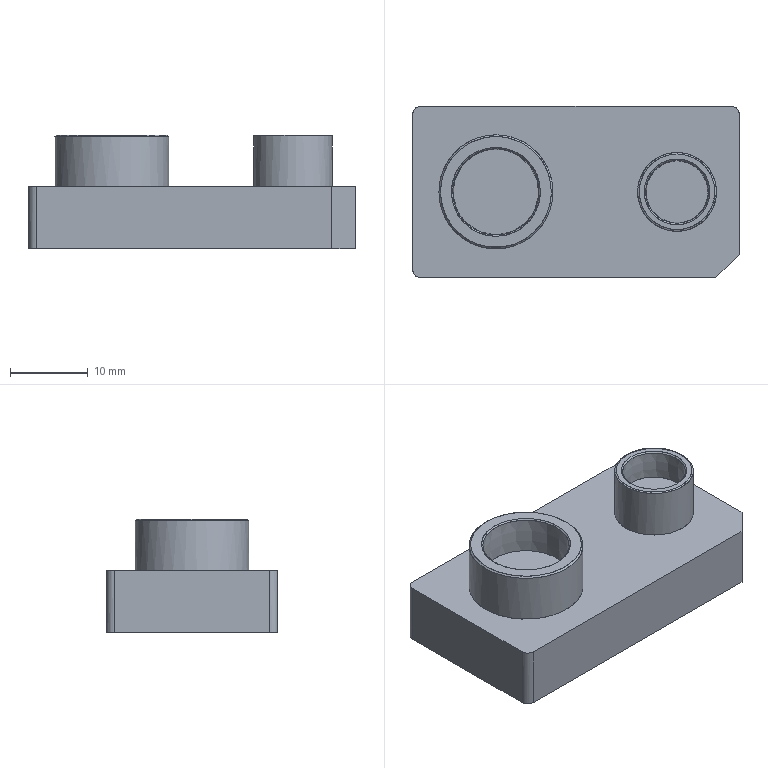NC program | PowerMill | posted by the shop | part box 42 x 22 x 14.621 mm
Lines 13250 to 14233 of 126517:
( TOOL ID   D10_1_1 )
( TOOL DIA. 10. TIP RAD 0 LENGTH 69.8 )
( Z = -.269 )
T3 M6
T14
G91 G28 Z0
G0 G90 G54
M08
S8500 M3
X0 Y0 M8
G43 Z11.801 H3
X-28.191 Y.483
Z.931
G1 Z-.269 F360
X-22.918 Y.327 F600
X-9.229 Y-12.572
G3 X-8.361 Y-12.468 I-1.292 J14.426
G1 X-8.126 Y-12.428
X-7.724 Y-12.351
X-7.405 Y-12.28
X-7.078 Y-12.198
X-6.754 Y-12.109
X-6.129 Y-11.908
X-5.492 Y-11.665
X-5.051 Y-11.472
X-4.855 Y-11.381
X-4.533 Y-11.219
X-21.847 Y5.097
X-21.746 Y5.321
X-21.544 Y5.734
X-21.428 Y5.955
X-21.195 Y6.374
X-21.109 Y6.516
X-20.794 Y7.013
X-20.47 Y7.475
X-20.089 Y7.968
X-19.835 Y8.267
X-19.487 Y8.652
X-1.123 Y-8.653
X-.713 Y-8.199
X-.395 Y-7.812
X-.268 Y-7.647
X-.032 Y-7.328
X.241 Y-6.93
X.403 Y-6.674
X.561 Y-6.416
X.766 Y-6.056
X.932 Y-5.738
X1.092 Y-5.416
X1.237 Y-5.099
X-16.078 Y11.219
X-15.693 Y11.408
X-15.371 Y11.557
X-14.797 Y11.792
X-14.418 Y11.927
X-14.1 Y12.034
X-13.782 Y12.128
X-13.463 Y12.216
X-13.143 Y12.294
X-12.821 Y12.365
X-12.184 Y12.478
X-11.547 Y12.557
X-11.379 Y12.57
X2.309 Y-.33
G0 Z4.001
G1 X28.324 Y-3.114 F10000
G0 Z.931
G1 Z-.269 F360
X23.158 Y-2.05 F600
X12.123 Y10.326
X11.843 Y10.299
X11.524 Y10.258
X11.204 Y10.207
X10.885 Y10.145
X10.566 Y10.074
X10.247 Y9.992
X9.919 Y9.895
X9.608 Y9.793
X9.289 Y9.677
X9.037 Y9.576
X8.65 Y9.408
X8.332 Y9.252
X8.012 Y9.085
X7.79 Y8.957
X21.303 Y-6.198
X21.1 Y-6.466
X20.782 Y-6.846
X20.622 Y-7.022
X20.314 Y-7.343
X20.145 Y-7.507
X19.824 Y-7.801
X19.609 Y-7.982
X19.205 Y-8.301
X18.866 Y-8.544
X18.547 Y-8.756
X18.211 Y-8.959
X4.696 Y6.199
X4.595 Y6.064
X4.374 Y5.744
X4.182 Y5.444
X3.98 Y5.106
X3.809 Y4.787
X3.648 Y4.467
X3.503 Y4.149
X3.369 Y3.829
X3.225 Y3.444
X3.139 Y3.191
X3.042 Y2.872
X2.955 Y2.552
X2.88 Y2.233
X2.842 Y2.05
X13.876 Y-10.326
G0 Z11.801
X0 Y0
Z9.801
X1.258 Y-21.755
Z-5.62
G1 Z-6.82 F360
Y-16.48 F600
X1.136 Y-5.545
X.851 Y-6.099
X.787 Y-6.215
X.451 Y-6.779
X.268 Y-7.062
X.073 Y-7.344
X-.284 Y-7.825
X-.581 Y-8.192
X-.827 Y-8.474
X-1.1 Y-8.77
X-1.418 Y-9.093
X-1.696 Y-9.356
X-1.974 Y-9.604
X-2.27 Y-9.853
X-2.674 Y-10.169
X-3.121 Y-10.49
X-3.491 Y-10.734
X-3.688 Y-10.857
X-4.255 Y-11.183
X-4.476 Y-11.299
X-4.823 Y-11.472
X-5.39 Y-11.726
X-5.735 Y-11.864
X-5.958 Y-11.947
X-6.525 Y-12.139
X-7.092 Y-12.301
X-7.66 Y-12.436
X-8.227 Y-12.543
X-8.795 Y-12.624
X-9.362 Y-12.679
X-9.929 Y-12.708
X-10.497 Y-12.712
X-11.064 Y-12.691
X-11.632 Y-12.644
X-12.199 Y-12.572
X-12.766 Y-12.473
X-12.98 Y-12.429
X-13.334 Y-12.348
X-13.901 Y-12.195
X-14.469 Y-12.013
X-14.874 Y-11.864
X-15.036 Y-11.8
X-15.603 Y-11.557
X-16.171 Y-11.28
X-16.738 Y-10.966
X-17.117 Y-10.734
X-17.305 Y-10.613
X-17.589 Y-10.42
X-17.935 Y-10.169
X-18.44 Y-9.77
X-18.697 Y-9.55
X-19.008 Y-9.268
X-19.245 Y-9.039
X-19.546 Y-8.731
X-19.782 Y-8.474
X-20.142 Y-8.053
X-20.477 Y-7.627
X-20.71 Y-7.305
X-21.06 Y-6.779
X-21.277 Y-6.422
X-21.396 Y-6.215
X-21.694 Y-5.65
X-21.829 Y-5.369
X-21.957 Y-5.085
X-22.188 Y-4.52
X-22.412 Y-3.879
X-22.558 Y-3.39
X-22.7 Y-2.825
X-22.816 Y-2.26
X-22.905 Y-1.695
X-22.968 Y-1.13
X-23.006 Y-.565
X-23.018 Y0
X-23.006 Y.565
X-22.968 Y1.13
X-22.905 Y1.695
X-22.816 Y2.26
X-22.7 Y2.825
X-22.558 Y3.39
X-22.388 Y3.955
X-22.188 Y4.52
X-21.957 Y5.085
X-21.829 Y5.369
X-21.694 Y5.65
X-21.396 Y6.215
X-21.277 Y6.422
X-21.06 Y6.779
X-20.682 Y7.344
X-20.477 Y7.627
X-20.142 Y8.053
X-19.782 Y8.474
X-19.546 Y8.731
X-19.245 Y9.039
X-19.008 Y9.268
X-18.635 Y9.604
X-18.44 Y9.77
X-17.873 Y10.216
X-17.589 Y10.42
X-17.305 Y10.613
X-17.117 Y10.734
X-16.738 Y10.966
X-16.133 Y11.299
X-15.603 Y11.557
X-15.036 Y11.801
X-14.874 Y11.864
X-14.469 Y12.013
X-13.901 Y12.195
X-13.334 Y12.348
X-12.98 Y12.429
X-12.766 Y12.473
X-12.199 Y12.572
X-11.632 Y12.645
X-11.064 Y12.691
X-10.497 Y12.712
X-9.929 Y12.708
X-9.362 Y12.679
X-8.795 Y12.624
X-8.227 Y12.543
X-7.63 Y12.429
X-7.092 Y12.301
X-6.525 Y12.139
X-5.958 Y11.948
X-5.735 Y11.864
X-5.39 Y11.726
X-4.823 Y11.472
X-4.476 Y11.299
X-4.255 Y11.183
X-3.688 Y10.857
X-3.491 Y10.734
X-3.121 Y10.49
X-2.674 Y10.169
X-2.27 Y9.853
X-1.974 Y9.604
X-1.696 Y9.356
X-1.364 Y9.039
X-1.1 Y8.77
X-.827 Y8.474
X-.581 Y8.192
X-.284 Y7.825
X.073 Y7.344
X.268 Y7.062
X.451 Y6.779
X.624 Y6.497
X.851 Y6.097
X1.085 Y5.65
G2 X1.418 Y4.921 I-11.182 J-5.554
G1 X1.579 Y4.52
X1.779 Y3.955
X1.949 Y3.39
X2.092 Y2.825
X2.207 Y2.26
X2.296 Y1.695
X2.359 Y1.13
X2.397 Y.565
X2.409 Y0
X2.397 Y-.565
X2.359 Y-1.13
X2.296 Y-1.695
X2.207 Y-2.26
X2.092 Y-2.825
X1.949 Y-3.39
X1.779 Y-3.955
X1.579 Y-4.52
X1.418 Y-4.921
X1.282 Y-5.235
X1.136 Y-5.545
X.548 Y-6.8
X.438 Y-6.998 Z-6.818
X.302 Y-7.178 Z-6.811
X-.628 Y-8.247 Z-6.755
X-.637 Y-8.257 Z-6.748
Z-6.727
X-.628 Y-8.246 Z-6.72
X-.581 Y-8.192 Z-6.721 F360
X-.35 Y-7.909 Z-6.728
X-.284 Y-7.825 Z-6.729
X.073 Y-7.344 Z-6.74
X.268 Y-7.062 Z-6.746
X.451 Y-6.779 Z-6.752
X.787 Y-6.215 Z-6.763
X.851 Y-6.099 Z-6.766
X1.085 Y-5.65 Z-6.774
X1.258 Y-5.288 Z-6.781
X1.418 Y-4.921 Z-6.788
X1.579 Y-4.52 Z-6.796
X1.779 Y-3.955 Z-6.806
X1.949 Y-3.39 Z-6.817
X1.986 Y-3.254 Z-6.819
X1.997 Y-3.207 Z-6.82
X3.536 Y-4.437 F600
X3.443 Y-4.237
X3.323 Y-3.955
X3.111 Y-3.39
X2.935 Y-2.825
X2.793 Y-2.26
X2.735 Y-1.977
X2.685 Y-1.695
X2.642 Y-1.412
X2.608 Y-1.13
X2.562 Y-.565
X2.553 Y-.377
X2.546 Y0
X2.553 Y.377
X2.562 Y.565
X2.608 Y1.13
X2.642 Y1.412
X2.685 Y1.695
X2.735 Y1.977
X2.793 Y2.26
X2.935 Y2.825
X3.121 Y3.417
X3.323 Y3.955
X3.443 Y4.237
X3.574 Y4.52
X3.714 Y4.802
X3.866 Y5.085
X4.029 Y5.367
X4.255 Y5.728
X4.382 Y5.916
X4.594 Y6.215
X4.823 Y6.512
X5.043 Y6.779
X5.39 Y7.167
X5.561 Y7.344
X5.958 Y7.726
X6.165 Y7.909
X6.525 Y8.207
X6.809 Y8.423
X7.092 Y8.624
X7.376 Y8.812
X7.749 Y9.039
X8.227 Y9.301
X8.511 Y9.441
X8.873 Y9.604
X9.362 Y9.8
X9.929 Y9.993
X10.578 Y10.169
X11.064 Y10.273
X11.632 Y10.364
X12.199 Y10.423
X12.766 Y10.451
X13.334 Y10.448
X13.901 Y10.415
X14.469 Y10.35
X15.036 Y10.254
X15.422 Y10.169
X15.603 Y10.125
X15.887 Y10.047
X16.171 Y9.961
X16.738 Y9.762
X17.127 Y9.604
X17.305 Y9.526
X17.589 Y9.393
X17.873 Y9.249
X18.251 Y9.039
X18.44 Y8.926
X18.724 Y8.748
X19.121 Y8.474
X19.264 Y8.369
X19.575 Y8.127
X19.859 Y7.889
X20.142 Y7.633
X20.439 Y7.344
X20.71 Y7.06
X20.957 Y6.779
X21.199 Y6.485
X21.406 Y6.215
X21.607 Y5.932
X21.845 Y5.572
X22.134 Y5.085
X22.285 Y4.802
X22.426 Y4.52
X22.677 Y3.955
X22.889 Y3.39
X22.979 Y3.112
X23.065 Y2.825
X23.207 Y2.26
X23.265 Y1.977
X23.315 Y1.695
X23.358 Y1.412
X23.392 Y1.13
X23.438 Y.565
X23.454 Y0
X23.438 Y-.565
X23.392 Y-1.13
X23.358 Y-1.412
X23.315 Y-1.695
X23.265 Y-1.977
X23.207 Y-2.26
X23.065 Y-2.825
X22.979 Y-3.112
X22.889 Y-3.39
X22.677 Y-3.955
X22.557 Y-4.237
X22.426 Y-4.52
X22.285 Y-4.802
X22.134 Y-5.085
X21.845 Y-5.573
X21.607 Y-5.932
X21.406 Y-6.215
X21.277 Y-6.385
X20.957 Y-6.779
X20.708 Y-7.062
X20.439 Y-7.344
X20.142 Y-7.633
X19.835 Y-7.909
X19.575 Y-8.127
X19.348 Y-8.306
X19.008 Y-8.555
X18.724 Y-8.747
X18.44 Y-8.926
X18.251 Y-9.039
X17.873 Y-9.249
X17.589 Y-9.393
X17.305 Y-9.526
X17.128 Y-9.604
X16.738 Y-9.762
X16.454 Y-9.867
X16.172 Y-9.961
X15.887 Y-10.047
X15.603 Y-10.125
X15.422 Y-10.169
X15.036 Y-10.254
X14.469 Y-10.35
X13.901 Y-10.415
X13.334 Y-10.448
X13.05 Y-10.454
X12.766 Y-10.451
X12.199 Y-10.423
X11.632 Y-10.364
X11.064 Y-10.273
X10.497 Y-10.15
X9.929 Y-9.993
X9.362 Y-9.8
X8.795 Y-9.571
X8.511 Y-9.441
X8.227 Y-9.301
X7.749 Y-9.039
X7.376 Y-8.812
X7.092 Y-8.624
X6.809 Y-8.423
X6.525 Y-8.207
X6.165 Y-7.909
X5.958 Y-7.726
X5.561 Y-7.344
X5.39 Y-7.167
X5.043 Y-6.779
X4.823 Y-6.513
X4.594 Y-6.215
X4.42 Y-5.971
X4.204 Y-5.65
X4.029 Y-5.367
X3.866 Y-5.085
X3.714 Y-4.802
X3.536 Y-4.437
G0 Z9.801
X0 Y0
X25.992 Y-17.264
Z-13.52
G1 Z-14.72 F360
G3 X22.456 Y-13.728 I-1.768 J1.768 F600
G1 X21.585 Y-14.599
X21.584 Y-14.6
X21.583 Y-14.601
X21.395 Y-14.779
X21.393 Y-14.78
X21.392 Y-14.782
X21.232 Y-14.919
X21.23 Y-14.921
X21.229 Y-14.922
X21.073 Y-15.045
X21.072 Y-15.046
X21.07 Y-15.047
X20.797 Y-15.24
X20.795 Y-15.242
X20.792 Y-15.244
X20.433 Y-15.46
X20.43 Y-15.461
X20.428 Y-15.462
X20.234 Y-15.562
X20.233 Y-15.563
X20.232
X20.109 Y-15.621
X20.108 Y-15.622
X20.106 Y-15.623
X19.79 Y-15.754
X19.787 Y-15.755
X19.784 Y-15.756
X19.4 Y-15.883
X19.397 Y-15.884
X19.395 Y-15.885
X19.147 Y-15.949
X19.145
X19.142 Y-15.95
X18.826 Y-16.012
X18.824 Y-16.013
X18.821
X18.505 Y-16.055
X18.502
X18.5
X18.184 Y-16.077
X18.181
X18.179
X17.863 Y-16.08
X17.862
X-20.075 Y-16.079
X-20.077
X-20.078
X-20.394 Y-16.067
X-20.397
X-20.399
X-20.715 Y-16.038
X-20.717 Y-16.037
X-20.719
X-21.035 Y-15.991
X-21.037
X-21.039 Y-15.99
X-21.356 Y-15.927
X-21.358 Y-15.926
X-21.36
X-21.676 Y-15.844
X-21.678
X-21.68 Y-15.843
X-21.996 Y-15.743
X-21.998 Y-15.742
X-22.001 Y-15.741
X-22.317 Y-15.621
X-22.319 Y-15.62
X-22.321
X-22.637 Y-15.478
X-22.639 Y-15.477
X-22.641 Y-15.476
X-22.957 Y-15.312
X-22.959 Y-15.311
X-22.96
X-23.076 Y-15.244
X-23.077
X-23.078 Y-15.243
X-23.279 Y-15.12
X-23.28 Y-15.119
X-23.282 Y-15.118
X-23.565 Y-14.925
X-23.567 Y-14.923
X-23.569 Y-14.922
X-23.918 Y-14.649
X-23.921 Y-14.647
X-23.923 Y-14.645
X-24.239 Y-14.359
X-24.24 Y-14.357
X-24.241 Y-14.356
X-24.315 Y-14.283
X-24.316 Y-14.282
X-24.317 Y-14.281
X-24.56 Y-14.022
X-24.562 Y-14.02
X-24.563 Y-14.018
X-24.866 Y-13.645
X-24.868 Y-13.642
X-24.87 Y-13.64
X-25.09 Y-13.324
X-25.091 Y-13.322
X-25.092 Y-13.321
X-25.201 Y-13.149
X-25.202 Y-13.147
X-25.203 Y-13.146
X-25.287 Y-13.002
X-25.288 Y-13.001
X-25.289 Y-12.999
X-25.456 Y-12.683
X-25.457 Y-12.681
X-25.458 Y-12.679
X-25.602 Y-12.363
X-25.603 Y-12.361
X-25.604 Y-12.359
X-25.727 Y-12.042
Y-12.04
X-25.728 Y-12.038
X-25.831 Y-11.722
X-25.832 Y-11.72
Y-11.718
X-25.916 Y-11.402
X-25.917 Y-11.4
Y-11.397
X-25.982 Y-11.081
X-25.983 Y-11.079
Y-11.077
X-26.032 Y-10.761
Y-10.759
X-26.033 Y-10.757
X-26.063 Y-10.441
X-26.064 Y-10.439
Y-10.437
X-26.079 Y-10.12
Y-10.119
Y-10.117
X-26.08 Y-9.801
Y9.801
X-26.079 Y10.117
Y10.119
Y10.12
X-26.064 Y10.436
Y10.439
Y10.441
X-26.033 Y10.757
X-26.032 Y10.759
Y10.761
X-25.984 Y11.077
X-25.983 Y11.079
Y11.081
X-25.917 Y11.398
Y11.4
X-25.916 Y11.402
X-25.843 Y11.68
Y11.682
X-25.842 Y11.684
X-25.728 Y12.038
X-25.727 Y12.04
X-25.726 Y12.042
X-25.604 Y12.359
X-25.603 Y12.36
X-25.602 Y12.362
X-25.523 Y12.542
X-25.522 Y12.543
Y12.545
X-25.457 Y12.68
X-25.456 Y12.682
Y12.683
X-25.289 Y12.999
X-25.288 Y13.001
X-25.287 Y13.002
X-25.203 Y13.146
X-25.202 Y13.147
X-25.201 Y13.148
X-25.093 Y13.321
X-25.092 Y13.322
X-25.091 Y13.324
X-24.883 Y13.622
X-24.882 Y13.624
X-24.88 Y13.626
X-24.613 Y13.96
X-24.611 Y13.963
X-24.609 Y13.965
X-24.317 Y14.281
X-24.316 Y14.282
X-24.315 Y14.283
X-24.241 Y14.356
X-24.24 Y14.357
X-24.239 Y14.358
X-23.973 Y14.602
X-23.971 Y14.604
X-23.969 Y14.605
X-23.603 Y14.898
X-23.6 Y14.899
X-23.598 Y14.901
X-23.282 Y15.118
X-23.28 Y15.119
X-23.279 Y15.12
X-23.078 Y15.243
X-23.077 Y15.244
X-23.076
X-22.96 Y15.311
X-22.959
X-22.957 Y15.312
X-22.641 Y15.476
X-22.639 Y15.477
X-22.637 Y15.478
X-22.321 Y15.62
X-22.319
X-22.317 Y15.621
X-22.001 Y15.741
X-21.998 Y15.742
X-21.996 Y15.743
X-21.68 Y15.843
X-21.678 Y15.844
X-21.676
X-21.36 Y15.926
X-21.358
X-21.355 Y15.927
X-21.039 Y15.99
X-21.037
X-21.035
X-20.719 Y16.037
X-20.717 Y16.038
X-20.715
X-20.399 Y16.066
X-20.397
X-20.395
X-20.079 Y16.079
X-20.077
X-20.075
X-.158
X20.075
X20.077
X20.078
X20.394 Y16.067
X20.397
X20.399
X20.715 Y16.038
X20.717 Y16.037
X20.719
X21.035 Y15.991
X21.037
X21.039 Y15.99
X21.356 Y15.927
X21.358 Y15.926
X21.36
X21.676 Y15.844
X21.678
X21.68 Y15.843
X21.996 Y15.743
X21.998 Y15.742
X22.001 Y15.741
X22.317 Y15.621
X22.319 Y15.62
X22.321
X22.637 Y15.478
X22.639 Y15.477
X22.641 Y15.476
X22.957 Y15.312
X22.959 Y15.311
X22.96
X23.076 Y15.244
X23.077
X23.078 Y15.243
X23.279 Y15.12
X23.28 Y15.119
X23.282 Y15.118
X23.565 Y14.925
X23.567 Y14.923
X23.569 Y14.922
X23.918 Y14.649
X23.921 Y14.647
X23.923 Y14.645
X24.239 Y14.359
X24.24 Y14.357
X24.241 Y14.356
X24.315 Y14.283
X24.316 Y14.282
X24.317 Y14.281
X24.56 Y14.022
X24.562 Y14.02
X24.563 Y14.018
X24.866 Y13.645
X24.868 Y13.642
X24.87 Y13.64
X25.09 Y13.324
X25.091 Y13.322
X25.092 Y13.321
X25.201 Y13.149
X25.202 Y13.147
X25.203 Y13.146
X25.287 Y13.002
X25.288 Y13.001
X25.289 Y12.999
X25.456 Y12.683
X25.457 Y12.681
X25.458 Y12.679
X25.602 Y12.363
X25.603 Y12.361
X25.604 Y12.359
X25.727 Y12.042
Y12.04
X25.728 Y12.038
X25.831 Y11.722
X25.832 Y11.72
Y11.718
X25.916 Y11.402
X25.917 Y11.4
Y11.397
X25.982 Y11.081
X25.983 Y11.079
Y11.077
X26.032 Y10.761
Y10.759
X26.033 Y10.757
X26.063 Y10.441
X26.064 Y10.439
Y10.437
X26.079 Y10.12
Y10.119
Y10.117
X26.08 Y9.801
Y-7.904
Y-7.905
X26.075 Y-8.221
Y-8.223
Y-8.226
X26.051 Y-8.542
Y-8.545
X26.05 Y-8.547
X26.006 Y-8.863
Y-8.866
X26.005 Y-8.868
X25.94 Y-9.184
X25.939 Y-9.187
Y-9.189
X25.852 Y-9.506
X25.851 Y-9.508
X25.85 Y-9.511
X25.74 Y-9.827
X25.739 Y-9.829
X25.738 Y-9.832
X25.603 Y-10.148
Y-10.15
X25.602 Y-10.152
X25.522 Y-10.316
X25.521 Y-10.317
X25.52 Y-10.318
X25.439 Y-10.471
X25.438 Y-10.472
X25.437 Y-10.474
X25.245 Y-10.79
X25.243 Y-10.793
X25.242 Y-10.796
X25.015 Y-11.112
X25.014 Y-11.114
X25.013 Y-11.115
X24.88 Y-11.279
X24.879 Y-11.281
X24.877 Y-11.282
X24.743 Y-11.434
X24.742 Y-11.435
X24.741 Y-11.437
X24.559 Y-11.625
X24.558 Y-11.626
X22.456 Y-13.728
G3 X25.992 Y-17.264 I1.768 J-1.768
G1 X25.94 Y-17.202
G3 X22.405 Y-13.666 I-1.768 J1.768
G1 X21.528 Y-14.543
X21.34 Y-14.721
X21.18 Y-14.859
X21.024 Y-14.982
X20.751 Y-15.175
X20.391 Y-15.391
X20.198 Y-15.491
X20.075 Y-15.549
X19.759 Y-15.68
X19.375 Y-15.807
X19.127 Y-15.871
X18.811 Y-15.934
X18.495 Y-15.975
X18.178 Y-15.997
X17.862 Y-16.
X-19.443
X-20.075 Y-15.999
X-20.391 Y-15.987
X-20.708 Y-15.958
X-21.024 Y-15.912
X-21.34 Y-15.848
X-21.656 Y-15.767
X-21.972 Y-15.667
X-22.288 Y-15.547
X-22.604 Y-15.405
X-22.921 Y-15.241
X-23.036 Y-15.175
X-23.237 Y-15.052
X-23.52 Y-14.859
X-23.869 Y-14.586
X-24.185 Y-14.299
X-24.259 Y-14.227
X-24.501 Y-13.967
X-24.804 Y-13.594
X-25.025 Y-13.278
X-25.134 Y-13.106
X-25.218 Y-12.962
X-25.385 Y-12.646
X-25.529 Y-12.33
X-25.652 Y-12.014
X-25.755 Y-11.697
X-25.839 Y-11.381
X-25.904 Y-11.065
X-25.953 Y-10.749
X-25.984 Y-10.433
X-25.999 Y-10.117
X-26. Y-9.801
Y9.801
X-25.999 Y10.117
X-25.984 Y10.433
X-25.953 Y10.749
X-25.905 Y11.065
X-25.839 Y11.381
X-25.766 Y11.659
X-25.652 Y12.014
X-25.529 Y12.33
X-25.45 Y12.51
X-25.385 Y12.646
X-25.218 Y12.962
X-25.134 Y13.106
X-25.025 Y13.278
X-24.817 Y13.577
X-24.551 Y13.91
X-24.259 Y14.227
X-24.185 Y14.299
X-23.919 Y14.543
X-23.553 Y14.835
X-23.237 Y15.052
X-23.036 Y15.175
X-22.921 Y15.241
X-22.604 Y15.405
X-22.288 Y15.547
X-21.972 Y15.667
X-21.656 Y15.767
X-21.34 Y15.848
X-21.024 Y15.911
X-20.708 Y15.958
X-20.391 Y15.986
X-20.075 Y15.999
X-19.759 Y16.
X-.158
X19.443
X20.075 Y15.999
X20.391 Y15.987
X20.708 Y15.958
X21.024 Y15.912
X21.34 Y15.848
X21.656 Y15.767
X21.972 Y15.667
X22.288 Y15.547
X22.604 Y15.405
X22.921 Y15.241
X23.036 Y15.175
X23.237 Y15.052
X23.52 Y14.859
X23.869 Y14.586
X24.185 Y14.299
X24.259 Y14.227
X24.501 Y13.967
X24.804 Y13.594
X25.025 Y13.278
X25.134 Y13.106
X25.218 Y12.962
X25.385 Y12.646
X25.529 Y12.33
X25.652 Y12.014
X25.755 Y11.697
X25.839 Y11.381
X25.904 Y11.065
X25.953 Y10.749
X25.984 Y10.433
X25.999 Y10.117
X26. Y9.801
Y-7.904
X25.995 Y-8.22
X25.971 Y-8.536
X25.927 Y-8.852
X25.862 Y-9.168
X25.775 Y-9.484
X25.665 Y-9.801
X25.53 Y-10.117
X25.45 Y-10.28
X25.368 Y-10.433
X25.177 Y-10.749
X24.95 Y-11.065
X24.817 Y-11.229
X24.683 Y-11.381
X24.501 Y-11.57
X22.405 Y-13.666
G3 X25.94 Y-17.202 I1.768 J-1.768
G0 Z9.801
Z10.801
X0 Y0
M9
M5
M01